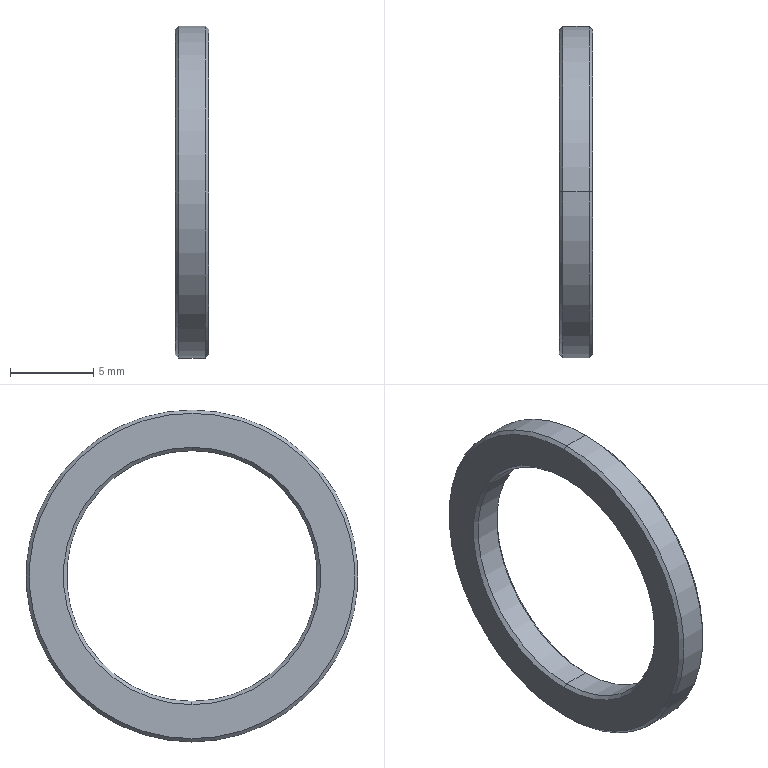Part | SolidWorks | features Chamfer 1, Extrusion 1 | 1 solid | 14 faces | box 2 x 20 x 20 mm | volume 265.75 mm3 | cone 8 | cylinder 4 | plane 2 | commonest cylinder face diameters 15.1 x2 20 x2
STEP:
#1=CARTESIAN_POINT('',(2.,0.,-9.8));
#2=VERTEX_POINT('',#1);
#3=CARTESIAN_POINT('',(2.,0.,9.8));
#4=VERTEX_POINT('',#3);
#5=CARTESIAN_POINT('',(2.,0.,0.));
#6=DIRECTION('',(1.,0.,0.));
#7=DIRECTION('',(0.,0.,-1.));
#8=AXIS2_PLACEMENT_3D('',#5,#6,#7);
#9=CIRCLE('',#8,9.8);
#10=EDGE_CURVE('',#2,#4,#9,.T.);
#11=ORIENTED_EDGE('',*,*,#10,.F.);
#12=CARTESIAN_POINT('',(1.8,0.,-10.));
#13=VERTEX_POINT('',#12);
#14=CARTESIAN_POINT('',(2.,0.,-9.8));
#15=DIRECTION('',(-0.7071,0.,-0.7071));
#16=VECTOR('',#15,1000.);
#17=LINE('',#14,#16);
#18=EDGE_CURVE('',#2,#13,#17,.T.);
#19=ORIENTED_EDGE('',*,*,#18,.T.);
#20=CARTESIAN_POINT('',(1.8,0.,10.));
#21=VERTEX_POINT('',#20);
#22=CARTESIAN_POINT('',(1.8,0.,0.));
#23=DIRECTION('',(-1.,0.,0.));
#24=DIRECTION('',(0.,0.,-1.));
#25=AXIS2_PLACEMENT_3D('',#22,#23,#24);
#26=CIRCLE('',#25,10.);
#27=EDGE_CURVE('',#21,#13,#26,.T.);
#28=ORIENTED_EDGE('',*,*,#27,.F.);
#29=CARTESIAN_POINT('',(2.,0.,9.8));
#30=DIRECTION('',(-0.7071,0.,0.7071));
#31=VECTOR('',#30,1000.);
#32=LINE('',#29,#31);
#33=EDGE_CURVE('',#4,#21,#32,.T.);
#34=ORIENTED_EDGE('',*,*,#33,.F.);
#35=EDGE_LOOP('',(#11,#19,#28,#34));
#36=FACE_OUTER_BOUND('',#35,.T.);
#37=CARTESIAN_POINT('',(2.,0.,0.));
#38=DIRECTION('',(-1.,0.,0.));
#39=DIRECTION('',(0.,0.,1.));
#40=AXIS2_PLACEMENT_3D('',#37,#38,#39);
#41=CONICAL_SURFACE('',#40,9.8,0.7854);
#42=ADVANCED_FACE('',(#36),#41,.T.);
#43=CARTESIAN_POINT('',(1.8,0.,7.55));
#44=VERTEX_POINT('',#43);
#45=CARTESIAN_POINT('',(1.8,0.,-7.55));
#46=VERTEX_POINT('',#45);
#47=CARTESIAN_POINT('',(1.8,0.,0.));
#48=DIRECTION('',(1.,0.,0.));
#49=DIRECTION('',(0.,0.,-1.));
#50=AXIS2_PLACEMENT_3D('',#47,#48,#49);
#51=CIRCLE('',#50,7.55);
#52=EDGE_CURVE('',#44,#46,#51,.T.);
#53=ORIENTED_EDGE('',*,*,#52,.F.);
#54=CARTESIAN_POINT('',(2.,0.,7.75));
#55=VERTEX_POINT('',#54);
#56=CARTESIAN_POINT('',(1.8,0.,7.55));
#57=DIRECTION('',(0.7071,0.,0.7071));
#58=VECTOR('',#57,1000.);
#59=LINE('',#56,#58);
#60=EDGE_CURVE('',#44,#55,#59,.T.);
#61=ORIENTED_EDGE('',*,*,#60,.T.);
#62=CARTESIAN_POINT('',(2.,0.,-7.75));
#63=VERTEX_POINT('',#62);
#64=CARTESIAN_POINT('',(2.,0.,0.));
#65=DIRECTION('',(-1.,0.,0.));
#66=DIRECTION('',(0.,0.,-1.));
#67=AXIS2_PLACEMENT_3D('',#64,#65,#66);
#68=CIRCLE('',#67,7.75);
#69=EDGE_CURVE('',#63,#55,#68,.T.);
#70=ORIENTED_EDGE('',*,*,#69,.F.);
#71=CARTESIAN_POINT('',(1.8,0.,-7.55));
#72=DIRECTION('',(0.7071,0.,-0.7071));
#73=VECTOR('',#72,1000.);
#74=LINE('',#71,#73);
#75=EDGE_CURVE('',#46,#63,#74,.T.);
#76=ORIENTED_EDGE('',*,*,#75,.F.);
#77=EDGE_LOOP('',(#53,#61,#70,#76));
#78=FACE_OUTER_BOUND('',#77,.T.);
#79=CARTESIAN_POINT('',(1.8,0.,0.));
#80=DIRECTION('',(1.,0.,0.));
#81=DIRECTION('',(0.,0.,-1.));
#82=AXIS2_PLACEMENT_3D('',#79,#80,#81);
#83=CONICAL_SURFACE('',#82,7.55,0.7854);
#84=ADVANCED_FACE('',(#78),#83,.F.);
#85=CARTESIAN_POINT('',(0.,0.,9.8));
#86=VERTEX_POINT('',#85);
#87=CARTESIAN_POINT('',(0.,0.,-9.8));
#88=VERTEX_POINT('',#87);
#89=CARTESIAN_POINT('',(0.,0.,0.));
#90=DIRECTION('',(-1.,0.,0.));
#91=DIRECTION('',(0.,0.,-1.));
#92=AXIS2_PLACEMENT_3D('',#89,#90,#91);
#93=CIRCLE('',#92,9.8);
#94=EDGE_CURVE('',#86,#88,#93,.T.);
#95=ORIENTED_EDGE('',*,*,#94,.F.);
#96=CARTESIAN_POINT('',(0.2,0.,10.));
#97=VERTEX_POINT('',#96);
#98=CARTESIAN_POINT('',(0.2,0.,10.));
#99=DIRECTION('',(0.7071,0.,0.7071));
#100=VECTOR('',#99,1000.);
#101=LINE('',#98,#100);
#102=EDGE_CURVE('',#86,#97,#101,.T.);
#103=ORIENTED_EDGE('',*,*,#102,.T.);
#104=CARTESIAN_POINT('',(0.2,0.,-10.));
#105=VERTEX_POINT('',#104);
#106=CARTESIAN_POINT('',(0.2,0.,0.));
#107=DIRECTION('',(1.,0.,0.));
#108=DIRECTION('',(0.,0.,-1.));
#109=AXIS2_PLACEMENT_3D('',#106,#107,#108);
#110=CIRCLE('',#109,10.);
#111=EDGE_CURVE('',#105,#97,#110,.T.);
#112=ORIENTED_EDGE('',*,*,#111,.F.);
#113=CARTESIAN_POINT('',(0.2,0.,-10.));
#114=DIRECTION('',(0.7071,0.,-0.7071));
#115=VECTOR('',#114,1000.);
#116=LINE('',#113,#115);
#117=EDGE_CURVE('',#88,#105,#116,.T.);
#118=ORIENTED_EDGE('',*,*,#117,.F.);
#119=EDGE_LOOP('',(#95,#103,#112,#118));
#120=FACE_OUTER_BOUND('',#119,.T.);
#121=CARTESIAN_POINT('',(0.2,0.,0.));
#122=DIRECTION('',(1.,0.,0.));
#123=DIRECTION('',(0.,0.,-1.));
#124=AXIS2_PLACEMENT_3D('',#121,#122,#123);
#125=CONICAL_SURFACE('',#124,10.,0.7854);
#126=ADVANCED_FACE('',(#120),#125,.T.);
#127=CARTESIAN_POINT('',(0.2,0.,-7.55));
#128=VERTEX_POINT('',#127);
#129=CARTESIAN_POINT('',(0.2,0.,7.55));
#130=VERTEX_POINT('',#129);
#131=CARTESIAN_POINT('',(0.2,0.,0.));
#132=DIRECTION('',(-1.,0.,0.));
#133=DIRECTION('',(0.,0.,-1.));
#134=AXIS2_PLACEMENT_3D('',#131,#132,#133);
#135=CIRCLE('',#134,7.55);
#136=EDGE_CURVE('',#128,#130,#135,.T.);
#137=ORIENTED_EDGE('',*,*,#136,.F.);
#138=CARTESIAN_POINT('',(0.,0.,-7.75));
#139=VERTEX_POINT('',#138);
#140=CARTESIAN_POINT('',(0.,0.,-7.75));
#141=DIRECTION('',(-0.7071,0.,-0.7071));
#142=VECTOR('',#141,1000.);
#143=LINE('',#140,#142);
#144=EDGE_CURVE('',#128,#139,#143,.T.);
#145=ORIENTED_EDGE('',*,*,#144,.T.);
#146=CARTESIAN_POINT('',(0.,0.,7.75));
#147=VERTEX_POINT('',#146);
#148=CARTESIAN_POINT('',(0.,0.,0.));
#149=DIRECTION('',(1.,0.,0.));
#150=DIRECTION('',(0.,0.,-1.));
#151=AXIS2_PLACEMENT_3D('',#148,#149,#150);
#152=CIRCLE('',#151,7.75);
#153=EDGE_CURVE('',#147,#139,#152,.T.);
#154=ORIENTED_EDGE('',*,*,#153,.F.);
#155=CARTESIAN_POINT('',(0.,0.,7.75));
#156=DIRECTION('',(-0.7071,0.,0.7071));
#157=VECTOR('',#156,1000.);
#158=LINE('',#155,#157);
#159=EDGE_CURVE('',#130,#147,#158,.T.);
#160=ORIENTED_EDGE('',*,*,#159,.F.);
#161=EDGE_LOOP('',(#137,#145,#154,#160));
#162=FACE_OUTER_BOUND('',#161,.T.);
#163=CARTESIAN_POINT('',(0.,0.,0.));
#164=DIRECTION('',(-1.,0.,0.));
#165=DIRECTION('',(0.,0.,1.));
#166=AXIS2_PLACEMENT_3D('',#163,#164,#165);
#167=CONICAL_SURFACE('',#166,7.75,0.7854);
#168=ADVANCED_FACE('',(#162),#167,.F.);
#169=ORIENTED_EDGE('',*,*,#52,.T.);
#170=CARTESIAN_POINT('',(2.,0.,-7.55));
#171=DIRECTION('',(-1.,0.,0.));
#172=VECTOR('',#171,1000.);
#173=LINE('',#170,#172);
#174=EDGE_CURVE('',#46,#128,#173,.T.);
#175=ORIENTED_EDGE('',*,*,#174,.T.);
#176=ORIENTED_EDGE('',*,*,#136,.T.);
#177=CARTESIAN_POINT('',(2.,0.,7.55));
#178=DIRECTION('',(-1.,0.,0.));
#179=VECTOR('',#178,1000.);
#180=LINE('',#177,#179);
#181=EDGE_CURVE('',#44,#130,#180,.T.);
#182=ORIENTED_EDGE('',*,*,#181,.F.);
#183=EDGE_LOOP('',(#169,#175,#176,#182));
#184=FACE_OUTER_BOUND('',#183,.T.);
#185=CARTESIAN_POINT('',(2.,0.,0.));
#186=DIRECTION('',(-1.,0.,0.));
#187=DIRECTION('',(0.,0.,1.));
#188=AXIS2_PLACEMENT_3D('',#185,#186,#187);
#189=CYLINDRICAL_SURFACE('',#188,7.55);
#190=ADVANCED_FACE('',(#184),#189,.F.);
#191=ORIENTED_EDGE('',*,*,#27,.T.);
#192=CARTESIAN_POINT('',(2.,0.,-10.));
#193=DIRECTION('',(-1.,0.,0.));
#194=VECTOR('',#193,1000.);
#195=LINE('',#192,#194);
#196=EDGE_CURVE('',#13,#105,#195,.T.);
#197=ORIENTED_EDGE('',*,*,#196,.T.);
#198=ORIENTED_EDGE('',*,*,#111,.T.);
#199=CARTESIAN_POINT('',(2.,0.,10.));
#200=DIRECTION('',(-1.,0.,0.));
#201=VECTOR('',#200,1000.);
#202=LINE('',#199,#201);
#203=EDGE_CURVE('',#21,#97,#202,.T.);
#204=ORIENTED_EDGE('',*,*,#203,.F.);
#205=EDGE_LOOP('',(#191,#197,#198,#204));
#206=FACE_OUTER_BOUND('',#205,.T.);
#207=CARTESIAN_POINT('',(2.,0.,0.));
#208=DIRECTION('',(-1.,0.,0.));
#209=DIRECTION('',(0.,0.,1.));
#210=AXIS2_PLACEMENT_3D('',#207,#208,#209);
#211=CYLINDRICAL_SURFACE('',#210,10.);
#212=ADVANCED_FACE('',(#206),#211,.T.);
#213=ORIENTED_EDGE('',*,*,#69,.T.);
#214=CARTESIAN_POINT('',(2.,0.,0.));
#215=DIRECTION('',(-1.,0.,0.));
#216=DIRECTION('',(0.,0.,-1.));
#217=AXIS2_PLACEMENT_3D('',#214,#215,#216);
#218=CIRCLE('',#217,7.75);
#219=EDGE_CURVE('',#55,#63,#218,.T.);
#220=ORIENTED_EDGE('',*,*,#219,.T.);
#221=EDGE_LOOP('',(#213,#220));
#222=FACE_BOUND('',#221,.T.);
#223=CARTESIAN_POINT('',(2.,0.,0.));
#224=DIRECTION('',(1.,0.,0.));
#225=DIRECTION('',(0.,0.,-1.));
#226=AXIS2_PLACEMENT_3D('',#223,#224,#225);
#227=CIRCLE('',#226,9.8);
#228=EDGE_CURVE('',#4,#2,#227,.T.);
#229=ORIENTED_EDGE('',*,*,#228,.T.);
#230=ORIENTED_EDGE('',*,*,#10,.T.);
#231=EDGE_LOOP('',(#229,#230));
#232=FACE_OUTER_BOUND('',#231,.T.);
#233=CARTESIAN_POINT('',(2.,0.,0.));
#234=DIRECTION('',(1.,0.,0.));
#235=DIRECTION('',(0.,0.,-1.));
#236=AXIS2_PLACEMENT_3D('',#233,#234,#235);
#237=PLANE('',#236);
#238=ADVANCED_FACE('',(#222,#232),#237,.T.);
#239=ORIENTED_EDGE('',*,*,#153,.T.);
#240=CARTESIAN_POINT('',(0.,0.,0.));
#241=DIRECTION('',(1.,0.,0.));
#242=DIRECTION('',(0.,0.,-1.));
#243=AXIS2_PLACEMENT_3D('',#240,#241,#242);
#244=CIRCLE('',#243,7.75);
#245=EDGE_CURVE('',#139,#147,#244,.T.);
#246=ORIENTED_EDGE('',*,*,#245,.T.);
#247=EDGE_LOOP('',(#239,#246));
#248=FACE_BOUND('',#247,.T.);
#249=CARTESIAN_POINT('',(0.,0.,0.));
#250=DIRECTION('',(-1.,0.,0.));
#251=DIRECTION('',(0.,0.,-1.));
#252=AXIS2_PLACEMENT_3D('',#249,#250,#251);
#253=CIRCLE('',#252,9.8);
#254=EDGE_CURVE('',#88,#86,#253,.T.);
#255=ORIENTED_EDGE('',*,*,#254,.T.);
#256=ORIENTED_EDGE('',*,*,#94,.T.);
#257=EDGE_LOOP('',(#255,#256));
#258=FACE_OUTER_BOUND('',#257,.T.);
#259=CARTESIAN_POINT('',(0.,0.,0.));
#260=DIRECTION('',(1.,0.,0.));
#261=DIRECTION('',(0.,0.,-1.));
#262=AXIS2_PLACEMENT_3D('',#259,#260,#261);
#263=PLANE('',#262);
#264=ADVANCED_FACE('',(#248,#258),#263,.F.);
#265=ORIENTED_EDGE('',*,*,#196,.F.);
#266=CARTESIAN_POINT('',(1.8,0.,0.));
#267=DIRECTION('',(-1.,0.,0.));
#268=DIRECTION('',(0.,0.,-1.));
#269=AXIS2_PLACEMENT_3D('',#266,#267,#268);
#270=CIRCLE('',#269,10.);
#271=EDGE_CURVE('',#13,#21,#270,.T.);
#272=ORIENTED_EDGE('',*,*,#271,.T.);
#273=ORIENTED_EDGE('',*,*,#203,.T.);
#274=CARTESIAN_POINT('',(0.2,0.,0.));
#275=DIRECTION('',(1.,0.,0.));
#276=DIRECTION('',(0.,0.,-1.));
#277=AXIS2_PLACEMENT_3D('',#274,#275,#276);
#278=CIRCLE('',#277,10.);
#279=EDGE_CURVE('',#97,#105,#278,.T.);
#280=ORIENTED_EDGE('',*,*,#279,.T.);
#281=EDGE_LOOP('',(#265,#272,#273,#280));
#282=FACE_OUTER_BOUND('',#281,.T.);
#283=CARTESIAN_POINT('',(2.,0.,0.));
#284=DIRECTION('',(-1.,0.,0.));
#285=DIRECTION('',(0.,0.,1.));
#286=AXIS2_PLACEMENT_3D('',#283,#284,#285);
#287=CYLINDRICAL_SURFACE('',#286,10.);
#288=ADVANCED_FACE('',(#282),#287,.T.);
#289=ORIENTED_EDGE('',*,*,#174,.F.);
#290=CARTESIAN_POINT('',(1.8,0.,0.));
#291=DIRECTION('',(1.,0.,0.));
#292=DIRECTION('',(0.,0.,-1.));
#293=AXIS2_PLACEMENT_3D('',#290,#291,#292);
#294=CIRCLE('',#293,7.55);
#295=EDGE_CURVE('',#46,#44,#294,.T.);
#296=ORIENTED_EDGE('',*,*,#295,.T.);
#297=ORIENTED_EDGE('',*,*,#181,.T.);
#298=CARTESIAN_POINT('',(0.2,0.,0.));
#299=DIRECTION('',(-1.,0.,0.));
#300=DIRECTION('',(0.,0.,-1.));
#301=AXIS2_PLACEMENT_3D('',#298,#299,#300);
#302=CIRCLE('',#301,7.55);
#303=EDGE_CURVE('',#130,#128,#302,.T.);
#304=ORIENTED_EDGE('',*,*,#303,.T.);
#305=EDGE_LOOP('',(#289,#296,#297,#304));
#306=FACE_OUTER_BOUND('',#305,.T.);
#307=CARTESIAN_POINT('',(2.,0.,0.));
#308=DIRECTION('',(-1.,0.,0.));
#309=DIRECTION('',(0.,0.,1.));
#310=AXIS2_PLACEMENT_3D('',#307,#308,#309);
#311=CYLINDRICAL_SURFACE('',#310,7.55);
#312=ADVANCED_FACE('',(#306),#311,.F.);
#313=ORIENTED_EDGE('',*,*,#144,.F.);
#314=ORIENTED_EDGE('',*,*,#303,.F.);
#315=ORIENTED_EDGE('',*,*,#159,.T.);
#316=ORIENTED_EDGE('',*,*,#245,.F.);
#317=EDGE_LOOP('',(#313,#314,#315,#316));
#318=FACE_OUTER_BOUND('',#317,.T.);
#319=CARTESIAN_POINT('',(0.,0.,0.));
#320=DIRECTION('',(-1.,0.,0.));
#321=DIRECTION('',(0.,0.,1.));
#322=AXIS2_PLACEMENT_3D('',#319,#320,#321);
#323=CONICAL_SURFACE('',#322,7.75,0.7854);
#324=ADVANCED_FACE('',(#318),#323,.F.);
#325=ORIENTED_EDGE('',*,*,#102,.F.);
#326=ORIENTED_EDGE('',*,*,#254,.F.);
#327=ORIENTED_EDGE('',*,*,#117,.T.);
#328=ORIENTED_EDGE('',*,*,#279,.F.);
#329=EDGE_LOOP('',(#325,#326,#327,#328));
#330=FACE_OUTER_BOUND('',#329,.T.);
#331=CARTESIAN_POINT('',(0.2,0.,0.));
#332=DIRECTION('',(1.,0.,0.));
#333=DIRECTION('',(0.,0.,-1.));
#334=AXIS2_PLACEMENT_3D('',#331,#332,#333);
#335=CONICAL_SURFACE('',#334,10.,0.7854);
#336=ADVANCED_FACE('',(#330),#335,.T.);
#337=ORIENTED_EDGE('',*,*,#60,.F.);
#338=ORIENTED_EDGE('',*,*,#295,.F.);
#339=ORIENTED_EDGE('',*,*,#75,.T.);
#340=ORIENTED_EDGE('',*,*,#219,.F.);
#341=EDGE_LOOP('',(#337,#338,#339,#340));
#342=FACE_OUTER_BOUND('',#341,.T.);
#343=CARTESIAN_POINT('',(1.8,0.,0.));
#344=DIRECTION('',(1.,0.,0.));
#345=DIRECTION('',(0.,0.,-1.));
#346=AXIS2_PLACEMENT_3D('',#343,#344,#345);
#347=CONICAL_SURFACE('',#346,7.55,0.7854);
#348=ADVANCED_FACE('',(#342),#347,.F.);
#349=ORIENTED_EDGE('',*,*,#18,.F.);
#350=ORIENTED_EDGE('',*,*,#228,.F.);
#351=ORIENTED_EDGE('',*,*,#33,.T.);
#352=ORIENTED_EDGE('',*,*,#271,.F.);
#353=EDGE_LOOP('',(#349,#350,#351,#352));
#354=FACE_OUTER_BOUND('',#353,.T.);
#355=CARTESIAN_POINT('',(2.,0.,0.));
#356=DIRECTION('',(-1.,0.,0.));
#357=DIRECTION('',(0.,0.,1.));
#358=AXIS2_PLACEMENT_3D('',#355,#356,#357);
#359=CONICAL_SURFACE('',#358,9.8,0.7854);
#360=ADVANCED_FACE('',(#354),#359,.T.);
#361=CLOSED_SHELL('',(#42,#84,#126,#168,#190,#212,#238,#264,#288,#312,#324,#336,#348,#360));
#362=MANIFOLD_SOLID_BREP('',#361);
#363=CARTESIAN_POINT('',(0.,0.,0.));
#364=DIRECTION('',(0.,0.,1.));
#365=DIRECTION('',(1.,0.,0.));
#366=AXIS2_PLACEMENT_3D('',#363,#364,#365);
#367=(LENGTH_UNIT()NAMED_UNIT(*)SI_UNIT(.MILLI.,.METRE.));
#368=UNCERTAINTY_MEASURE_WITH_UNIT(LENGTH_MEASURE(0.00001),#367,'','');
#369=(NAMED_UNIT(*)PLANE_ANGLE_UNIT()SI_UNIT($,.RADIAN.));
#370=(NAMED_UNIT(*)SI_UNIT($,.STERADIAN.)SOLID_ANGLE_UNIT());
#371=(GEOMETRIC_REPRESENTATION_CONTEXT(3)GLOBAL_UNCERTAINTY_ASSIGNED_CONTEXT((#368))GLOBAL_UNIT_ASSIGNED_CONTEXT((#367,#369,#370))REPRESENTATION_CONTEXT('',''));
#372=ADVANCED_BREP_SHAPE_REPRESENTATION('',(#362,#366),#371);